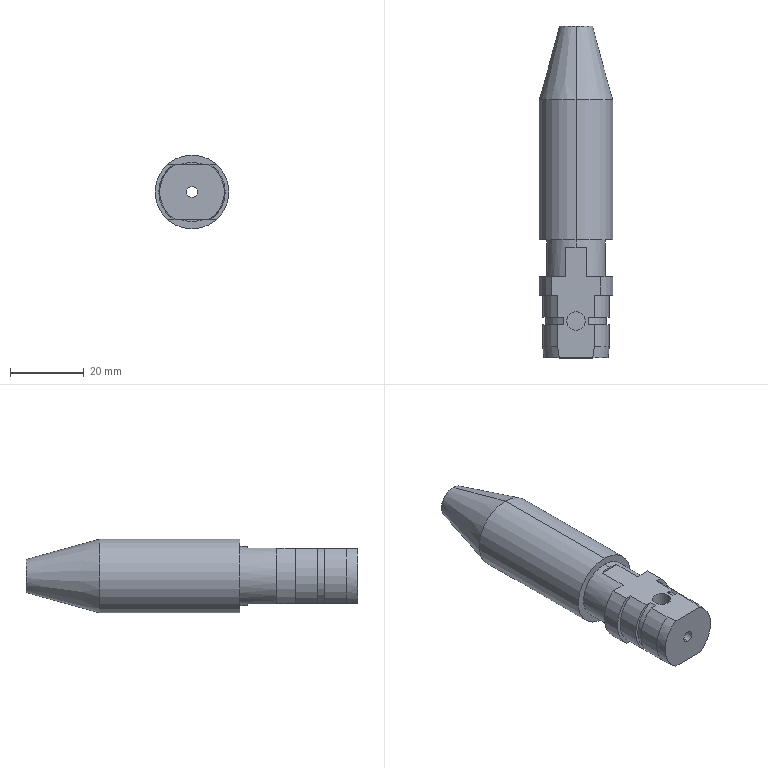Part | SolidWorks | features ICE 3, Revolution 1 | 1 solid | 39 faces | box 20 x 90 x 20 mm | volume 21802 mm3 | cylinder 18 | plane 17 | cone 4 | commonest cylinder face diameters 5 x4 18 x4 20 x4 3 x2 16 x2 16.4 x2
STEP:
#1=CARTESIAN_POINT('',(2.5,-35.854,-2.5));
#2=VERTEX_POINT('',#1);
#3=CARTESIAN_POINT('',(-2.5,-35.854,-2.5));
#4=VERTEX_POINT('',#3);
#5=CARTESIAN_POINT('',(0.,-35.854,-2.5));
#6=DIRECTION('',(0.,0.,-1.));
#7=DIRECTION('',(-1.,0.,0.));
#8=AXIS2_PLACEMENT_3D('',#5,#6,#7);
#9=CIRCLE('',#8,2.5);
#10=EDGE_CURVE('',#2,#4,#9,.T.);
#11=ORIENTED_EDGE('',*,*,#10,.F.);
#12=CARTESIAN_POINT('',(2.5,-35.854,-7.5));
#13=VERTEX_POINT('',#12);
#14=CARTESIAN_POINT('',(2.5,-35.854,-2.5));
#15=DIRECTION('',(0.,0.,-1.));
#16=VECTOR('',#15,1000.);
#17=LINE('',#14,#16);
#18=EDGE_CURVE('',#2,#13,#17,.T.);
#19=ORIENTED_EDGE('',*,*,#18,.T.);
#20=CARTESIAN_POINT('',(-2.5,-35.854,-7.5));
#21=VERTEX_POINT('',#20);
#22=CARTESIAN_POINT('',(0.,-35.854,-7.5));
#23=DIRECTION('',(0.,0.,-1.));
#24=DIRECTION('',(-1.,0.,0.));
#25=AXIS2_PLACEMENT_3D('',#22,#23,#24);
#26=CIRCLE('',#25,2.5);
#27=EDGE_CURVE('',#13,#21,#26,.T.);
#28=ORIENTED_EDGE('',*,*,#27,.T.);
#29=CARTESIAN_POINT('',(-2.5,-35.854,-2.5));
#30=DIRECTION('',(0.,0.,-1.));
#31=VECTOR('',#30,1000.);
#32=LINE('',#29,#31);
#33=EDGE_CURVE('',#4,#21,#32,.T.);
#34=ORIENTED_EDGE('',*,*,#33,.F.);
#35=EDGE_LOOP('',(#11,#19,#28,#34));
#36=FACE_OUTER_BOUND('',#35,.T.);
#37=CARTESIAN_POINT('',(0.,-35.854,-2.5));
#38=DIRECTION('',(0.,0.,-1.));
#39=DIRECTION('',(-1.,0.,0.));
#40=AXIS2_PLACEMENT_3D('',#37,#38,#39);
#41=CYLINDRICAL_SURFACE('',#40,2.5);
#42=ADVANCED_FACE('',(#36),#41,.F.);
#43=CARTESIAN_POINT('',(-2.5,-35.854,2.5));
#44=VERTEX_POINT('',#43);
#45=CARTESIAN_POINT('',(2.5,-35.854,2.5));
#46=VERTEX_POINT('',#45);
#47=CARTESIAN_POINT('',(0.,-35.854,2.5));
#48=DIRECTION('',(0.,0.,1.));
#49=DIRECTION('',(1.,0.,0.));
#50=AXIS2_PLACEMENT_3D('',#47,#48,#49);
#51=CIRCLE('',#50,2.5);
#52=EDGE_CURVE('',#44,#46,#51,.T.);
#53=ORIENTED_EDGE('',*,*,#52,.F.);
#54=CARTESIAN_POINT('',(-2.5,-35.854,7.5));
#55=VERTEX_POINT('',#54);
#56=CARTESIAN_POINT('',(-2.5,-35.854,2.5));
#57=DIRECTION('',(0.,0.,1.));
#58=VECTOR('',#57,1000.);
#59=LINE('',#56,#58);
#60=EDGE_CURVE('',#44,#55,#59,.T.);
#61=ORIENTED_EDGE('',*,*,#60,.T.);
#62=CARTESIAN_POINT('',(2.5,-35.854,7.5));
#63=VERTEX_POINT('',#62);
#64=CARTESIAN_POINT('',(0.,-35.854,7.5));
#65=DIRECTION('',(0.,0.,1.));
#66=DIRECTION('',(1.,0.,0.));
#67=AXIS2_PLACEMENT_3D('',#64,#65,#66);
#68=CIRCLE('',#67,2.5);
#69=EDGE_CURVE('',#55,#63,#68,.T.);
#70=ORIENTED_EDGE('',*,*,#69,.T.);
#71=CARTESIAN_POINT('',(2.5,-35.854,2.5));
#72=DIRECTION('',(0.,0.,1.));
#73=VECTOR('',#72,1000.);
#74=LINE('',#71,#73);
#75=EDGE_CURVE('',#46,#63,#74,.T.);
#76=ORIENTED_EDGE('',*,*,#75,.F.);
#77=EDGE_LOOP('',(#53,#61,#70,#76));
#78=FACE_OUTER_BOUND('',#77,.T.);
#79=CARTESIAN_POINT('',(0.,-35.854,2.5));
#80=DIRECTION('',(0.,0.,1.));
#81=DIRECTION('',(1.,0.,0.));
#82=AXIS2_PLACEMENT_3D('',#79,#80,#81);
#83=CYLINDRICAL_SURFACE('',#82,2.5);
#84=ADVANCED_FACE('',(#78),#83,.F.);
#85=CARTESIAN_POINT('',(0.,24.146,-10.));
#86=VERTEX_POINT('',#85);
#87=CARTESIAN_POINT('',(0.,24.146,10.));
#88=VERTEX_POINT('',#87);
#89=CARTESIAN_POINT('',(0.,24.146,0.));
#90=DIRECTION('',(0.,-1.,0.));
#91=DIRECTION('',(0.,0.,-1.));
#92=AXIS2_PLACEMENT_3D('',#89,#90,#91);
#93=CIRCLE('',#92,10.);
#94=EDGE_CURVE('',#86,#88,#93,.T.);
#95=ORIENTED_EDGE('',*,*,#94,.T.);
#96=CARTESIAN_POINT('',(0.,-13.854,10.));
#97=VERTEX_POINT('',#96);
#98=CARTESIAN_POINT('',(0.,0.,10.));
#99=DIRECTION('',(0.,-1.,0.));
#100=VECTOR('',#99,1000.);
#101=LINE('',#98,#100);
#102=EDGE_CURVE('',#88,#97,#101,.T.);
#103=ORIENTED_EDGE('',*,*,#102,.T.);
#104=CARTESIAN_POINT('',(0.,-13.854,-10.));
#105=VERTEX_POINT('',#104);
#106=CARTESIAN_POINT('',(0.,-13.854,0.));
#107=DIRECTION('',(0.,-1.,0.));
#108=DIRECTION('',(0.,0.,-1.));
#109=AXIS2_PLACEMENT_3D('',#106,#107,#108);
#110=CIRCLE('',#109,10.);
#111=EDGE_CURVE('',#105,#97,#110,.T.);
#112=ORIENTED_EDGE('',*,*,#111,.F.);
#113=CARTESIAN_POINT('',(0.,0.,-10.));
#114=DIRECTION('',(0.,-1.,0.));
#115=VECTOR('',#114,1000.);
#116=LINE('',#113,#115);
#117=EDGE_CURVE('',#86,#105,#116,.T.);
#118=ORIENTED_EDGE('',*,*,#117,.F.);
#119=EDGE_LOOP('',(#95,#103,#112,#118));
#120=FACE_OUTER_BOUND('',#119,.T.);
#121=CARTESIAN_POINT('',(0.,0.,0.));
#122=DIRECTION('',(0.,-1.,0.));
#123=DIRECTION('',(0.,0.,-1.));
#124=AXIS2_PLACEMENT_3D('',#121,#122,#123);
#125=CYLINDRICAL_SURFACE('',#124,10.);
#126=ADVANCED_FACE('',(#120),#125,.T.);
#127=CARTESIAN_POINT('',(0.,44.146,-4.5));
#128=VERTEX_POINT('',#127);
#129=CARTESIAN_POINT('',(0.,44.146,4.5));
#130=VERTEX_POINT('',#129);
#131=CARTESIAN_POINT('',(0.,44.146,0.));
#132=DIRECTION('',(0.,-1.,0.));
#133=DIRECTION('',(0.,0.,-1.));
#134=AXIS2_PLACEMENT_3D('',#131,#132,#133);
#135=CIRCLE('',#134,4.5);
#136=EDGE_CURVE('',#128,#130,#135,.T.);
#137=ORIENTED_EDGE('',*,*,#136,.T.);
#138=CARTESIAN_POINT('',(0.,44.146,4.5));
#139=DIRECTION('',(0.,-0.9642,0.2652));
#140=VECTOR('',#139,1000.);
#141=LINE('',#138,#140);
#142=EDGE_CURVE('',#130,#88,#141,.T.);
#143=ORIENTED_EDGE('',*,*,#142,.T.);
#144=ORIENTED_EDGE('',*,*,#94,.F.);
#145=CARTESIAN_POINT('',(0.,44.146,-4.5));
#146=DIRECTION('',(0.,-0.9642,-0.2652));
#147=VECTOR('',#146,1000.);
#148=LINE('',#145,#147);
#149=EDGE_CURVE('',#128,#86,#148,.T.);
#150=ORIENTED_EDGE('',*,*,#149,.F.);
#151=EDGE_LOOP('',(#137,#143,#144,#150));
#152=FACE_OUTER_BOUND('',#151,.T.);
#153=CARTESIAN_POINT('',(0.,44.146,0.));
#154=DIRECTION('',(0.,-1.,0.));
#155=DIRECTION('',(0.,0.,-1.));
#156=AXIS2_PLACEMENT_3D('',#153,#154,#155);
#157=CONICAL_SURFACE('',#156,4.5,0.2684);
#158=ADVANCED_FACE('',(#152),#157,.T.);
#159=CARTESIAN_POINT('',(0.,44.146,1.5));
#160=VERTEX_POINT('',#159);
#161=CARTESIAN_POINT('',(0.,44.146,-1.5));
#162=VERTEX_POINT('',#161);
#163=CARTESIAN_POINT('',(0.,44.146,0.));
#164=DIRECTION('',(0.,-1.,0.));
#165=DIRECTION('',(0.,0.,-1.));
#166=AXIS2_PLACEMENT_3D('',#163,#164,#165);
#167=CIRCLE('',#166,1.5);
#168=EDGE_CURVE('',#160,#162,#167,.T.);
#169=ORIENTED_EDGE('',*,*,#168,.F.);
#170=CARTESIAN_POINT('',(0.,-45.854,1.5));
#171=VERTEX_POINT('',#170);
#172=CARTESIAN_POINT('',(0.,0.,1.5));
#173=DIRECTION('',(0.,-1.,0.));
#174=VECTOR('',#173,1000.);
#175=LINE('',#172,#174);
#176=EDGE_CURVE('',#160,#171,#175,.T.);
#177=ORIENTED_EDGE('',*,*,#176,.T.);
#178=CARTESIAN_POINT('',(0.,-45.854,-1.5));
#179=VERTEX_POINT('',#178);
#180=CARTESIAN_POINT('',(0.,-45.854,0.));
#181=DIRECTION('',(0.,-1.,0.));
#182=DIRECTION('',(0.,0.,-1.));
#183=AXIS2_PLACEMENT_3D('',#180,#181,#182);
#184=CIRCLE('',#183,1.5);
#185=EDGE_CURVE('',#171,#179,#184,.T.);
#186=ORIENTED_EDGE('',*,*,#185,.T.);
#187=CARTESIAN_POINT('',(0.,0.,-1.5));
#188=DIRECTION('',(0.,-1.,0.));
#189=VECTOR('',#188,1000.);
#190=LINE('',#187,#189);
#191=EDGE_CURVE('',#162,#179,#190,.T.);
#192=ORIENTED_EDGE('',*,*,#191,.F.);
#193=EDGE_LOOP('',(#169,#177,#186,#192));
#194=FACE_OUTER_BOUND('',#193,.T.);
#195=CARTESIAN_POINT('',(0.,0.,0.));
#196=DIRECTION('',(0.,-1.,0.));
#197=DIRECTION('',(0.,0.,-1.));
#198=AXIS2_PLACEMENT_3D('',#195,#196,#197);
#199=CYLINDRICAL_SURFACE('',#198,1.5);
#200=ADVANCED_FACE('',(#194),#199,.F.);
#201=CARTESIAN_POINT('',(0.,-13.854,-8.));
#202=VERTEX_POINT('',#201);
#203=CARTESIAN_POINT('',(0.,-13.854,8.));
#204=VERTEX_POINT('',#203);
#205=CARTESIAN_POINT('',(0.,-13.854,0.));
#206=DIRECTION('',(0.,-1.,0.));
#207=DIRECTION('',(0.,0.,-1.));
#208=AXIS2_PLACEMENT_3D('',#205,#206,#207);
#209=CIRCLE('',#208,8.);
#210=EDGE_CURVE('',#202,#204,#209,.T.);
#211=ORIENTED_EDGE('',*,*,#210,.T.);
#212=CARTESIAN_POINT('',(0.,-15.854,8.));
#213=VERTEX_POINT('',#212);
#214=CARTESIAN_POINT('',(0.,0.,8.));
#215=DIRECTION('',(0.,-1.,0.));
#216=VECTOR('',#215,1000.);
#217=LINE('',#214,#216);
#218=EDGE_CURVE('',#204,#213,#217,.T.);
#219=ORIENTED_EDGE('',*,*,#218,.T.);
#220=CARTESIAN_POINT('',(2.784,-15.854,7.5));
#221=VERTEX_POINT('',#220);
#222=CARTESIAN_POINT('',(0.,-15.854,0.));
#223=DIRECTION('',(0.,-1.,0.));
#224=DIRECTION('',(0.,0.,-1.));
#225=AXIS2_PLACEMENT_3D('',#222,#223,#224);
#226=CIRCLE('',#225,8.);
#227=EDGE_CURVE('',#221,#213,#226,.T.);
#228=ORIENTED_EDGE('',*,*,#227,.F.);
#229=CARTESIAN_POINT('',(2.784,-23.854,7.5));
#230=VERTEX_POINT('',#229);
#231=CARTESIAN_POINT('',(2.784,0.,7.5));
#232=DIRECTION('',(0.,1.,0.));
#233=VECTOR('',#232,1000.);
#234=LINE('',#231,#233);
#235=EDGE_CURVE('',#230,#221,#234,.T.);
#236=ORIENTED_EDGE('',*,*,#235,.F.);
#237=CARTESIAN_POINT('',(2.784,-23.854,-7.5));
#238=VERTEX_POINT('',#237);
#239=CARTESIAN_POINT('',(0.,-23.854,0.));
#240=DIRECTION('',(0.,-1.,0.));
#241=DIRECTION('',(0.,0.,-1.));
#242=AXIS2_PLACEMENT_3D('',#239,#240,#241);
#243=CIRCLE('',#242,8.);
#244=EDGE_CURVE('',#238,#230,#243,.T.);
#245=ORIENTED_EDGE('',*,*,#244,.F.);
#246=CARTESIAN_POINT('',(2.784,-15.854,-7.5));
#247=VERTEX_POINT('',#246);
#248=CARTESIAN_POINT('',(2.784,0.,-7.5));
#249=DIRECTION('',(0.,-1.,0.));
#250=VECTOR('',#249,1000.);
#251=LINE('',#248,#250);
#252=EDGE_CURVE('',#247,#238,#251,.T.);
#253=ORIENTED_EDGE('',*,*,#252,.F.);
#254=CARTESIAN_POINT('',(0.,-15.854,-8.));
#255=VERTEX_POINT('',#254);
#256=CARTESIAN_POINT('',(0.,-15.854,0.));
#257=DIRECTION('',(0.,-1.,0.));
#258=DIRECTION('',(0.,0.,-1.));
#259=AXIS2_PLACEMENT_3D('',#256,#257,#258);
#260=CIRCLE('',#259,8.);
#261=EDGE_CURVE('',#255,#247,#260,.T.);
#262=ORIENTED_EDGE('',*,*,#261,.F.);
#263=CARTESIAN_POINT('',(0.,0.,-8.));
#264=DIRECTION('',(0.,-1.,0.));
#265=VECTOR('',#264,1000.);
#266=LINE('',#263,#265);
#267=EDGE_CURVE('',#202,#255,#266,.T.);
#268=ORIENTED_EDGE('',*,*,#267,.F.);
#269=EDGE_LOOP('',(#211,#219,#228,#236,#245,#253,#262,#268));
#270=FACE_OUTER_BOUND('',#269,.T.);
#271=CARTESIAN_POINT('',(0.,0.,0.));
#272=DIRECTION('',(0.,-1.,0.));
#273=DIRECTION('',(0.,0.,-1.));
#274=AXIS2_PLACEMENT_3D('',#271,#272,#273);
#275=CYLINDRICAL_SURFACE('',#274,8.);
#276=ADVANCED_FACE('',(#270),#275,.T.);
#277=CARTESIAN_POINT('',(0.,-45.854,0.));
#278=DIRECTION('',(0.,-1.,0.));
#279=DIRECTION('',(0.,0.,-1.));
#280=AXIS2_PLACEMENT_3D('',#277,#278,#279);
#281=CIRCLE('',#280,1.5);
#282=EDGE_CURVE('',#179,#171,#281,.T.);
#283=ORIENTED_EDGE('',*,*,#282,.F.);
#284=ORIENTED_EDGE('',*,*,#185,.F.);
#285=EDGE_LOOP('',(#283,#284));
#286=FACE_BOUND('',#285,.T.);
#287=CARTESIAN_POINT('',(-4.55,-45.854,-7.5));
#288=VERTEX_POINT('',#287);
#289=CARTESIAN_POINT('',(4.55,-45.854,-7.5));
#290=VERTEX_POINT('',#289);
#291=CARTESIAN_POINT('',(-13.155,-45.854,-7.5));
#292=DIRECTION('',(1.,0.,0.));
#293=VECTOR('',#292,1000.);
#294=LINE('',#291,#293);
#295=EDGE_CURVE('',#288,#290,#294,.T.);
#296=ORIENTED_EDGE('',*,*,#295,.T.);
#297=CARTESIAN_POINT('',(4.55,-45.854,7.5));
#298=VERTEX_POINT('',#297);
#299=CARTESIAN_POINT('',(0.,-45.854,0.));
#300=DIRECTION('',(0.,-1.,0.));
#301=DIRECTION('',(0.,0.,-1.));
#302=AXIS2_PLACEMENT_3D('',#299,#300,#301);
#303=CIRCLE('',#302,8.772);
#304=EDGE_CURVE('',#290,#298,#303,.T.);
#305=ORIENTED_EDGE('',*,*,#304,.T.);
#306=CARTESIAN_POINT('',(-4.55,-45.854,7.5));
#307=VERTEX_POINT('',#306);
#308=CARTESIAN_POINT('',(-13.155,-45.854,7.5));
#309=DIRECTION('',(-1.,0.,0.));
#310=VECTOR('',#309,1000.);
#311=LINE('',#308,#310);
#312=EDGE_CURVE('',#298,#307,#311,.T.);
#313=ORIENTED_EDGE('',*,*,#312,.T.);
#314=CARTESIAN_POINT('',(0.,-45.854,0.));
#315=DIRECTION('',(0.,-1.,0.));
#316=DIRECTION('',(0.,0.,-1.));
#317=AXIS2_PLACEMENT_3D('',#314,#315,#316);
#318=CIRCLE('',#317,8.772);
#319=EDGE_CURVE('',#307,#288,#318,.T.);
#320=ORIENTED_EDGE('',*,*,#319,.T.);
#321=EDGE_LOOP('',(#296,#305,#313,#320));
#322=FACE_OUTER_BOUND('',#321,.T.);
#323=CARTESIAN_POINT('',(-8.772,-45.854,0.));
#324=DIRECTION('',(0.,1.,0.));
#325=DIRECTION('',(0.,0.,1.));
#326=AXIS2_PLACEMENT_3D('',#323,#324,#325);
#327=PLANE('',#326);
#328=ADVANCED_FACE('',(#286,#322),#327,.F.);
#329=ORIENTED_EDGE('',*,*,#218,.F.);
#330=CARTESIAN_POINT('',(0.,-13.854,0.));
#331=DIRECTION('',(0.,-1.,0.));
#332=DIRECTION('',(0.,0.,-1.));
#333=AXIS2_PLACEMENT_3D('',#330,#331,#332);
#334=CIRCLE('',#333,8.);
#335=EDGE_CURVE('',#204,#202,#334,.T.);
#336=ORIENTED_EDGE('',*,*,#335,.T.);
#337=ORIENTED_EDGE('',*,*,#267,.T.);
#338=CARTESIAN_POINT('',(-2.784,-15.854,-7.5));
#339=VERTEX_POINT('',#338);
#340=CARTESIAN_POINT('',(0.,-15.854,0.));
#341=DIRECTION('',(0.,-1.,0.));
#342=DIRECTION('',(0.,0.,-1.));
#343=AXIS2_PLACEMENT_3D('',#340,#341,#342);
#344=CIRCLE('',#343,8.);
#345=EDGE_CURVE('',#339,#255,#344,.T.);
#346=ORIENTED_EDGE('',*,*,#345,.F.);
#347=CARTESIAN_POINT('',(-2.784,-23.854,-7.5));
#348=VERTEX_POINT('',#347);
#349=CARTESIAN_POINT('',(-2.784,0.,-7.5));
#350=DIRECTION('',(0.,1.,0.));
#351=VECTOR('',#350,1000.);
#352=LINE('',#349,#351);
#353=EDGE_CURVE('',#348,#339,#352,.T.);
#354=ORIENTED_EDGE('',*,*,#353,.F.);
#355=CARTESIAN_POINT('',(-2.784,-23.854,7.5));
#356=VERTEX_POINT('',#355);
#357=CARTESIAN_POINT('',(0.,-23.854,0.));
#358=DIRECTION('',(0.,-1.,0.));
#359=DIRECTION('',(0.,0.,-1.));
#360=AXIS2_PLACEMENT_3D('',#357,#358,#359);
#361=CIRCLE('',#360,8.);
#362=EDGE_CURVE('',#356,#348,#361,.T.);
#363=ORIENTED_EDGE('',*,*,#362,.F.);
#364=CARTESIAN_POINT('',(-2.784,-15.854,7.5));
#365=VERTEX_POINT('',#364);
#366=CARTESIAN_POINT('',(-2.784,0.,7.5));
#367=DIRECTION('',(0.,-1.,0.));
#368=VECTOR('',#367,1000.);
#369=LINE('',#366,#368);
#370=EDGE_CURVE('',#365,#356,#369,.T.);
#371=ORIENTED_EDGE('',*,*,#370,.F.);
#372=CARTESIAN_POINT('',(0.,-15.854,0.));
#373=DIRECTION('',(0.,-1.,0.));
#374=DIRECTION('',(0.,0.,-1.));
#375=AXIS2_PLACEMENT_3D('',#372,#373,#374);
#376=CIRCLE('',#375,8.);
#377=EDGE_CURVE('',#213,#365,#376,.T.);
#378=ORIENTED_EDGE('',*,*,#377,.F.);
#379=EDGE_LOOP('',(#329,#336,#337,#346,#354,#363,#371,#378));
#380=FACE_OUTER_BOUND('',#379,.T.);
#381=CARTESIAN_POINT('',(0.,0.,0.));
#382=DIRECTION('',(0.,-1.,0.));
#383=DIRECTION('',(0.,0.,-1.));
#384=AXIS2_PLACEMENT_3D('',#381,#382,#383);
#385=CYLINDRICAL_SURFACE('',#384,8.);
#386=ADVANCED_FACE('',(#380),#385,.T.);
#387=CARTESIAN_POINT('',(-6.614,-23.854,-7.5));
#388=VERTEX_POINT('',#387);
#389=CARTESIAN_POINT('',(-10.,-23.854,-7.5));
#390=DIRECTION('',(1.,0.,0.));
#391=VECTOR('',#390,1000.);
#392=LINE('',#389,#391);
#393=EDGE_CURVE('',#388,#348,#392,.T.);
#394=ORIENTED_EDGE('',*,*,#393,.F.);
#395=CARTESIAN_POINT('',(-6.614,-23.854,7.5));
#396=VERTEX_POINT('',#395);
#397=CARTESIAN_POINT('',(0.,-23.854,0.));
#398=DIRECTION('',(0.,-1.,0.));
#399=DIRECTION('',(0.,0.,-1.));
#400=AXIS2_PLACEMENT_3D('',#397,#398,#399);
#401=CIRCLE('',#400,10.);
#402=EDGE_CURVE('',#396,#388,#401,.T.);
#403=ORIENTED_EDGE('',*,*,#402,.F.);
#404=CARTESIAN_POINT('',(-10.,-23.854,7.5));
#405=DIRECTION('',(-1.,0.,0.));
#406=VECTOR('',#405,1000.);
#407=LINE('',#404,#406);
#408=EDGE_CURVE('',#356,#396,#407,.T.);
#409=ORIENTED_EDGE('',*,*,#408,.F.);
#410=ORIENTED_EDGE('',*,*,#362,.T.);
#411=EDGE_LOOP('',(#394,#403,#409,#410));
#412=FACE_OUTER_BOUND('',#411,.T.);
#413=CARTESIAN_POINT('',(-10.,-23.854,0.));
#414=DIRECTION('',(0.,-1.,0.));
#415=DIRECTION('',(0.,0.,-1.));
#416=AXIS2_PLACEMENT_3D('',#413,#414,#415);
#417=PLANE('',#416);
#418=ADVANCED_FACE('',(#412),#417,.F.);
#419=CARTESIAN_POINT('',(6.614,-23.854,-7.5));
#420=VERTEX_POINT('',#419);
#421=CARTESIAN_POINT('',(-10.,-23.854,-7.5));
#422=DIRECTION('',(1.,0.,0.));
#423=VECTOR('',#422,1000.);
#424=LINE('',#421,#423);
#425=EDGE_CURVE('',#238,#420,#424,.T.);
#426=ORIENTED_EDGE('',*,*,#425,.F.);
#427=ORIENTED_EDGE('',*,*,#244,.T.);
#428=CARTESIAN_POINT('',(6.614,-23.854,7.5));
#429=VERTEX_POINT('',#428);
#430=CARTESIAN_POINT('',(-10.,-23.854,7.5));
#431=DIRECTION('',(-1.,0.,0.));
#432=VECTOR('',#431,1000.);
#433=LINE('',#430,#432);
#434=EDGE_CURVE('',#429,#230,#433,.T.);
#435=ORIENTED_EDGE('',*,*,#434,.F.);
#436=CARTESIAN_POINT('',(0.,-23.854,0.));
#437=DIRECTION('',(0.,-1.,0.));
#438=DIRECTION('',(0.,0.,-1.));
#439=AXIS2_PLACEMENT_3D('',#436,#437,#438);
#440=CIRCLE('',#439,10.);
#441=EDGE_CURVE('',#420,#429,#440,.T.);
#442=ORIENTED_EDGE('',*,*,#441,.F.);
#443=EDGE_LOOP('',(#426,#427,#435,#442));
#444=FACE_OUTER_BOUND('',#443,.T.);
#445=CARTESIAN_POINT('',(-10.,-23.854,0.));
#446=DIRECTION('',(0.,-1.,0.));
#447=DIRECTION('',(0.,0.,-1.));
#448=AXIS2_PLACEMENT_3D('',#445,#446,#447);
#449=PLANE('',#448);
#450=ADVANCED_FACE('',(#444),#449,.F.);
#451=CARTESIAN_POINT('',(6.614,-28.854,-7.5));
#452=VERTEX_POINT('',#451);
#453=CARTESIAN_POINT('',(6.614,0.,-7.5));
#454=DIRECTION('',(0.,-1.,0.));
#455=VECTOR('',#454,1000.);
#456=LINE('',#453,#455);
#457=EDGE_CURVE('',#420,#452,#456,.T.);
#458=ORIENTED_EDGE('',*,*,#457,.F.);
#459=ORIENTED_EDGE('',*,*,#441,.T.);
#460=CARTESIAN_POINT('',(6.614,-28.854,7.5));
#461=VERTEX_POINT('',#460);
#462=CARTESIAN_POINT('',(6.614,0.,7.5));
#463=DIRECTION('',(0.,1.,0.));
#464=VECTOR('',#463,1000.);
#465=LINE('',#462,#464);
#466=EDGE_CURVE('',#461,#429,#465,.T.);
#467=ORIENTED_EDGE('',*,*,#466,.F.);
#468=CARTESIAN_POINT('',(0.,-28.854,0.));
#469=DIRECTION('',(0.,-1.,0.));
#470=DIRECTION('',(0.,0.,-1.));
#471=AXIS2_PLACEMENT_3D('',#468,#469,#470);
#472=CIRCLE('',#471,10.);
#473=EDGE_CURVE('',#452,#461,#472,.T.);
#474=ORIENTED_EDGE('',*,*,#473,.F.);
#475=EDGE_LOOP('',(#458,#459,#467,#474));
#476=FACE_OUTER_BOUND('',#475,.T.);
#477=CARTESIAN_POINT('',(0.,0.,0.));
#478=DIRECTION('',(0.,-1.,0.));
#479=DIRECTION('',(0.,0.,-1.));
#480=AXIS2_PLACEMENT_3D('',#477,#478,#479);
#481=CYLINDRICAL_SURFACE('',#480,10.);
#482=ADVANCED_FACE('',(#476),#481,.T.);
#483=CARTESIAN_POINT('',(-6.614,-28.854,-7.5));
#484=VERTEX_POINT('',#483);
#485=CARTESIAN_POINT('',(-6.614,0.,-7.5));
#486=DIRECTION('',(0.,1.,0.));
#487=VECTOR('',#486,1000.);
#488=LINE('',#485,#487);
#489=EDGE_CURVE('',#484,#388,#488,.T.);
#490=ORIENTED_EDGE('',*,*,#489,.F.);
#491=CARTESIAN_POINT('',(-6.614,-28.854,7.5));
#492=VERTEX_POINT('',#491);
#493=CARTESIAN_POINT('',(0.,-28.854,0.));
#494=DIRECTION('',(0.,-1.,0.));
#495=DIRECTION('',(0.,0.,-1.));
#496=AXIS2_PLACEMENT_3D('',#493,#494,#495);
#497=CIRCLE('',#496,10.);
#498=EDGE_CURVE('',#492,#484,#497,.T.);
#499=ORIENTED_EDGE('',*,*,#498,.F.);
#500=CARTESIAN_POINT('',(-6.614,0.,7.5));
#501=DIRECTION('',(0.,-1.,0.));
#502=VECTOR('',#501,1000.);
#503=LINE('',#500,#502);
#504=EDGE_CURVE('',#396,#492,#503,.T.);
#505=ORIENTED_EDGE('',*,*,#504,.F.);
#506=ORIENTED_EDGE('',*,*,#402,.T.);
#507=EDGE_LOOP('',(#490,#499,#505,#506));
#508=FACE_OUTER_BOUND('',#507,.T.);
#509=CARTESIAN_POINT('',(0.,0.,0.));
#510=DIRECTION('',(0.,-1.,0.));
#511=DIRECTION('',(0.,0.,-1.));
#512=AXIS2_PLACEMENT_3D('',#509,#510,#511);
#513=CYLINDRICAL_SURFACE('',#512,10.);
#514=ADVANCED_FACE('',(#508),#513,.T.);
#515=CARTESIAN_POINT('',(4.975,-28.854,-7.5));
#516=VERTEX_POINT('',#515);
#517=CARTESIAN_POINT('',(-10.,-28.854,-7.5));
#518=DIRECTION('',(-1.,0.,0.));
#519=VECTOR('',#518,1000.);
#520=LINE('',#517,#519);
#521=EDGE_CURVE('',#452,#516,#520,.T.);
#522=ORIENTED_EDGE('',*,*,#521,.F.);
#523=ORIENTED_EDGE('',*,*,#473,.T.);
#524=CARTESIAN_POINT('',(4.975,-28.854,7.5));
#525=VERTEX_POINT('',#524);
#526=CARTESIAN_POINT('',(-10.,-28.854,7.5));
#527=DIRECTION('',(1.,0.,0.));
#528=VECTOR('',#527,1000.);
#529=LINE('',#526,#528);
#530=EDGE_CURVE('',#525,#461,#529,.T.);
#531=ORIENTED_EDGE('',*,*,#530,.F.);
#532=CARTESIAN_POINT('',(0.,-28.854,0.));
#533=DIRECTION('',(0.,-1.,0.));
#534=DIRECTION('',(0.,0.,-1.));
#535=AXIS2_PLACEMENT_3D('',#532,#533,#534);
#536=CIRCLE('',#535,9.);
#537=EDGE_CURVE('',#516,#525,#536,.T.);
#538=ORIENTED_EDGE('',*,*,#537,.F.);
#539=EDGE_LOOP('',(#522,#523,#531,#538));
#540=FACE_OUTER_BOUND('',#539,.T.);
#541=CARTESIAN_POINT('',(-10.,-28.854,0.));
#542=DIRECTION('',(0.,1.,0.));
#543=DIRECTION('',(0.,0.,1.));
#544=AXIS2_PLACEMENT_3D('',#541,#542,#543);
#545=PLANE('',#544);
#546=ADVANCED_FACE('',(#540),#545,.F.);
#547=CARTESIAN_POINT('',(-4.975,-28.854,-7.5));
#548=VERTEX_POINT('',#547);
#549=CARTESIAN_POINT('',(-10.,-28.854,-7.5));
#550=DIRECTION('',(-1.,0.,0.));
#551=VECTOR('',#550,1000.);
#552=LINE('',#549,#551);
#553=EDGE_CURVE('',#548,#484,#552,.T.);
#554=ORIENTED_EDGE('',*,*,#553,.F.);
#555=CARTESIAN_POINT('',(-4.975,-28.854,7.5));
#556=VERTEX_POINT('',#555);
#557=CARTESIAN_POINT('',(0.,-28.854,0.));
#558=DIRECTION('',(0.,-1.,0.));
#559=DIRECTION('',(0.,0.,-1.));
#560=AXIS2_PLACEMENT_3D('',#557,#558,#559);
#561=CIRCLE('',#560,9.);
#562=EDGE_CURVE('',#556,#548,#561,.T.);
#563=ORIENTED_EDGE('',*,*,#562,.F.);
#564=CARTESIAN_POINT('',(-10.,-28.854,7.5));
#565=DIRECTION('',(1.,0.,0.));
#566=VECTOR('',#565,1000.);
#567=LINE('',#564,#566);
#568=EDGE_CURVE('',#492,#556,#567,.T.);
#569=ORIENTED_EDGE('',*,*,#568,.F.);
#570=ORIENTED_EDGE('',*,*,#498,.T.);
#571=EDGE_LOOP('',(#554,#563,#569,#570));
#572=FACE_OUTER_BOUND('',#571,.T.);
#573=CARTESIAN_POINT('',(-10.,-28.854,0.));
#574=DIRECTION('',(0.,1.,0.));
#575=DIRECTION('',(0.,0.,1.));
#576=AXIS2_PLACEMENT_3D('',#573,#574,#575);
#577=PLANE('',#576);
#578=ADVANCED_FACE('',(#572),#577,.F.);
#579=CARTESIAN_POINT('',(4.975,-34.854,-7.5));
#580=VERTEX_POINT('',#579);
#581=CARTESIAN_POINT('',(4.975,0.,-7.5));
#582=DIRECTION('',(0.,-1.,0.));
#583=VECTOR('',#582,1000.);
#584=LINE('',#581,#583);
#585=EDGE_CURVE('',#516,#580,#584,.T.);
#586=ORIENTED_EDGE('',*,*,#585,.F.);
#587=ORIENTED_EDGE('',*,*,#537,.T.);
#588=CARTESIAN_POINT('',(4.975,-34.854,7.5));
#589=VERTEX_POINT('',#588);
#590=CARTESIAN_POINT('',(4.975,0.,7.5));
#591=DIRECTION('',(0.,1.,0.));
#592=VECTOR('',#591,1000.);
#593=LINE('',#590,#592);
#594=EDGE_CURVE('',#589,#525,#593,.T.);
#595=ORIENTED_EDGE('',*,*,#594,.F.);
#596=CARTESIAN_POINT('',(0.,-34.854,0.));
#597=DIRECTION('',(0.,-1.,0.));
#598=DIRECTION('',(0.,0.,-1.));
#599=AXIS2_PLACEMENT_3D('',#596,#597,#598);
#600=CIRCLE('',#599,9.);
#601=EDGE_CURVE('',#580,#589,#600,.T.);
#602=ORIENTED_EDGE('',*,*,#601,.F.);
#603=EDGE_LOOP('',(#586,#587,#595,#602));
#604=FACE_OUTER_BOUND('',#603,.T.);
#605=CARTESIAN_POINT('',(0.,0.,0.));
#606=DIRECTION('',(0.,-1.,0.));
#607=DIRECTION('',(0.,0.,-1.));
#608=AXIS2_PLACEMENT_3D('',#605,#606,#607);
#609=CYLINDRICAL_SURFACE('',#608,9.);
#610=ADVANCED_FACE('',(#604),#609,.T.);
#611=CARTESIAN_POINT('',(-4.975,-34.854,-7.5));
#612=VERTEX_POINT('',#611);
#613=CARTESIAN_POINT('',(-4.975,0.,-7.5));
#614=DIRECTION('',(0.,1.,0.));
#615=VECTOR('',#614,1000.);
#616=LINE('',#613,#615);
#617=EDGE_CURVE('',#612,#548,#616,.T.);
#618=ORIENTED_EDGE('',*,*,#617,.F.);
#619=CARTESIAN_POINT('',(-4.975,-34.854,7.5));
#620=VERTEX_POINT('',#619);
#621=CARTESIAN_POINT('',(0.,-34.854,0.));
#622=DIRECTION('',(0.,-1.,0.));
#623=DIRECTION('',(0.,0.,-1.));
#624=AXIS2_PLACEMENT_3D('',#621,#622,#623);
#625=CIRCLE('',#624,9.);
#626=EDGE_CURVE('',#620,#612,#625,.T.);
#627=ORIENTED_EDGE('',*,*,#626,.F.);
#628=CARTESIAN_POINT('',(-4.975,0.,7.5));
#629=DIRECTION('',(0.,-1.,0.));
#630=VECTOR('',#629,1000.);
#631=LINE('',#628,#630);
#632=EDGE_CURVE('',#556,#620,#631,.T.);
#633=ORIENTED_EDGE('',*,*,#632,.F.);
#634=ORIENTED_EDGE('',*,*,#562,.T.);
#635=EDGE_LOOP('',(#618,#627,#633,#634));
#636=FACE_OUTER_BOUND('',#635,.T.);
#637=CARTESIAN_POINT('',(0.,0.,0.));
#638=DIRECTION('',(0.,-1.,0.));
#639=DIRECTION('',(0.,0.,-1.));
#640=AXIS2_PLACEMENT_3D('',#637,#638,#639);
#641=CYLINDRICAL_SURFACE('',#640,9.);
#642=ADVANCED_FACE('',(#636),#641,.T.);
#643=CARTESIAN_POINT('',(3.315,-34.854,-7.5));
#644=VERTEX_POINT('',#643);
#645=CARTESIAN_POINT('',(-9.,-34.854,-7.5));
#646=DIRECTION('',(-1.,0.,0.));
#647=VECTOR('',#646,1000.);
#648=LINE('',#645,#647);
#649=EDGE_CURVE('',#580,#644,#648,.T.);
#650=ORIENTED_EDGE('',*,*,#649,.F.);
#651=ORIENTED_EDGE('',*,*,#601,.T.);
#652=CARTESIAN_POINT('',(3.315,-34.854,7.5));
#653=VERTEX_POINT('',#652);
#654=CARTESIAN_POINT('',(-9.,-34.854,7.5));
#655=DIRECTION('',(1.,0.,0.));
#656=VECTOR('',#655,1000.);
#657=LINE('',#654,#656);
#658=EDGE_CURVE('',#653,#589,#657,.T.);
#659=ORIENTED_EDGE('',*,*,#658,.F.);
#660=CARTESIAN_POINT('',(0.,-34.854,0.));
#661=DIRECTION('',(0.,-1.,0.));
#662=DIRECTION('',(0.,0.,-1.));
#663=AXIS2_PLACEMENT_3D('',#660,#661,#662);
#664=CIRCLE('',#663,8.2);
#665=EDGE_CURVE('',#644,#653,#664,.T.);
#666=ORIENTED_EDGE('',*,*,#665,.F.);
#667=EDGE_LOOP('',(#650,#651,#659,#666));
#668=FACE_OUTER_BOUND('',#667,.T.);
#669=CARTESIAN_POINT('',(-9.,-34.854,0.));
#670=DIRECTION('',(0.,1.,0.));
#671=DIRECTION('',(0.,0.,1.));
#672=AXIS2_PLACEMENT_3D('',#669,#670,#671);
#673=PLANE('',#672);
#674=ADVANCED_FACE('',(#668),#673,.F.);
#675=CARTESIAN_POINT('',(-3.315,-34.854,-7.5));
#676=VERTEX_POINT('',#675);
#677=CARTESIAN_POINT('',(-9.,-34.854,-7.5));
#678=DIRECTION('',(-1.,0.,0.));
#679=VECTOR('',#678,1000.);
#680=LINE('',#677,#679);
#681=EDGE_CURVE('',#676,#612,#680,.T.);
#682=ORIENTED_EDGE('',*,*,#681,.F.);
#683=CARTESIAN_POINT('',(-3.315,-34.854,7.5));
#684=VERTEX_POINT('',#683);
#685=CARTESIAN_POINT('',(0.,-34.854,0.));
#686=DIRECTION('',(0.,-1.,0.));
#687=DIRECTION('',(0.,0.,-1.));
#688=AXIS2_PLACEMENT_3D('',#685,#686,#687);
#689=CIRCLE('',#688,8.2);
#690=EDGE_CURVE('',#684,#676,#689,.T.);
#691=ORIENTED_EDGE('',*,*,#690,.F.);
#692=CARTESIAN_POINT('',(-9.,-34.854,7.5));
#693=DIRECTION('',(1.,0.,0.));
#694=VECTOR('',#693,1000.);
#695=LINE('',#692,#694);
#696=EDGE_CURVE('',#620,#684,#695,.T.);
#697=ORIENTED_EDGE('',*,*,#696,.F.);
#698=ORIENTED_EDGE('',*,*,#626,.T.);
#699=EDGE_LOOP('',(#682,#691,#697,#698));
#700=FACE_OUTER_BOUND('',#699,.T.);
#701=CARTESIAN_POINT('',(-9.,-34.854,0.));
#702=DIRECTION('',(0.,1.,0.));
#703=DIRECTION('',(0.,0.,1.));
#704=AXIS2_PLACEMENT_3D('',#701,#702,#703);
#705=PLANE('',#704);
#706=ADVANCED_FACE('',(#700),#705,.F.);
#707=CARTESIAN_POINT('',(3.315,-36.854,-7.5));
#708=VERTEX_POINT('',#707);
#709=CARTESIAN_POINT('',(3.315,0.,-7.5));
#710=DIRECTION('',(0.,-1.,0.));
#711=VECTOR('',#710,1000.);
#712=LINE('',#709,#711);
#713=EDGE_CURVE('',#644,#708,#712,.T.);
#714=ORIENTED_EDGE('',*,*,#713,.F.);
#715=ORIENTED_EDGE('',*,*,#665,.T.);
#716=CARTESIAN_POINT('',(3.315,-36.854,7.5));
#717=VERTEX_POINT('',#716);
#718=CARTESIAN_POINT('',(3.315,0.,7.5));
#719=DIRECTION('',(0.,1.,0.));
#720=VECTOR('',#719,1000.);
#721=LINE('',#718,#720);
#722=EDGE_CURVE('',#717,#653,#721,.T.);
#723=ORIENTED_EDGE('',*,*,#722,.F.);
#724=CARTESIAN_POINT('',(0.,-36.854,0.));
#725=DIRECTION('',(0.,-1.,0.));
#726=DIRECTION('',(0.,0.,-1.));
#727=AXIS2_PLACEMENT_3D('',#724,#725,#726);
#728=CIRCLE('',#727,8.2);
#729=EDGE_CURVE('',#708,#717,#728,.T.);
#730=ORIENTED_EDGE('',*,*,#729,.F.);
#731=EDGE_LOOP('',(#714,#715,#723,#730));
#732=FACE_OUTER_BOUND('',#731,.T.);
#733=CARTESIAN_POINT('',(0.,0.,0.));
#734=DIRECTION('',(0.,-1.,0.));
#735=DIRECTION('',(0.,0.,-1.));
#736=AXIS2_PLACEMENT_3D('',#733,#734,#735);
#737=CYLINDRICAL_SURFACE('',#736,8.2);
#738=ADVANCED_FACE('',(#732),#737,.T.);
#739=CARTESIAN_POINT('',(-3.315,-36.854,-7.5));
#740=VERTEX_POINT('',#739);
#741=CARTESIAN_POINT('',(-3.315,0.,-7.5));
#742=DIRECTION('',(0.,1.,0.));
#743=VECTOR('',#742,1000.);
#744=LINE('',#741,#743);
#745=EDGE_CURVE('',#740,#676,#744,.T.);
#746=ORIENTED_EDGE('',*,*,#745,.F.);
#747=CARTESIAN_POINT('',(-3.315,-36.854,7.5));
#748=VERTEX_POINT('',#747);
#749=CARTESIAN_POINT('',(0.,-36.854,0.));
#750=DIRECTION('',(0.,-1.,0.));
#751=DIRECTION('',(0.,0.,-1.));
#752=AXIS2_PLACEMENT_3D('',#749,#750,#751);
#753=CIRCLE('',#752,8.2);
#754=EDGE_CURVE('',#748,#740,#753,.T.);
#755=ORIENTED_EDGE('',*,*,#754,.F.);
#756=CARTESIAN_POINT('',(-3.315,0.,7.5));
#757=DIRECTION('',(0.,-1.,0.));
#758=VECTOR('',#757,1000.);
#759=LINE('',#756,#758);
#760=EDGE_CURVE('',#684,#748,#759,.T.);
#761=ORIENTED_EDGE('',*,*,#760,.F.);
#762=ORIENTED_EDGE('',*,*,#690,.T.);
#763=EDGE_LOOP('',(#746,#755,#761,#762));
#764=FACE_OUTER_BOUND('',#763,.T.);
#765=CARTESIAN_POINT('',(0.,0.,0.));
#766=DIRECTION('',(0.,-1.,0.));
#767=DIRECTION('',(0.,0.,-1.));
#768=AXIS2_PLACEMENT_3D('',#765,#766,#767);
#769=CYLINDRICAL_SURFACE('',#768,8.2);
#770=ADVANCED_FACE('',(#764),#769,.T.);
#771=CARTESIAN_POINT('',(-4.975,-36.854,-7.5));
#772=VERTEX_POINT('',#771);
#773=CARTESIAN_POINT('',(-9.,-36.854,-7.5));
#774=DIRECTION('',(1.,0.,0.));
#775=VECTOR('',#774,1000.);
#776=LINE('',#773,#775);
#777=EDGE_CURVE('',#772,#740,#776,.T.);
#778=ORIENTED_EDGE('',*,*,#777,.F.);
#779=CARTESIAN_POINT('',(-4.975,-36.854,7.5));
#780=VERTEX_POINT('',#779);
#781=CARTESIAN_POINT('',(0.,-36.854,0.));
#782=DIRECTION('',(0.,-1.,0.));
#783=DIRECTION('',(0.,0.,-1.));
#784=AXIS2_PLACEMENT_3D('',#781,#782,#783);
#785=CIRCLE('',#784,9.);
#786=EDGE_CURVE('',#780,#772,#785,.T.);
#787=ORIENTED_EDGE('',*,*,#786,.F.);
#788=CARTESIAN_POINT('',(-9.,-36.854,7.5));
#789=DIRECTION('',(-1.,0.,0.));
#790=VECTOR('',#789,1000.);
#791=LINE('',#788,#790);
#792=EDGE_CURVE('',#748,#780,#791,.T.);
#793=ORIENTED_EDGE('',*,*,#792,.F.);
#794=ORIENTED_EDGE('',*,*,#754,.T.);
#795=EDGE_LOOP('',(#778,#787,#793,#794));
#796=FACE_OUTER_BOUND('',#795,.T.);
#797=CARTESIAN_POINT('',(-9.,-36.854,0.));
#798=DIRECTION('',(0.,-1.,0.));
#799=DIRECTION('',(0.,0.,-1.));
#800=AXIS2_PLACEMENT_3D('',#797,#798,#799);
#801=PLANE('',#800);
#802=ADVANCED_FACE('',(#796),#801,.F.);
#803=CARTESIAN_POINT('',(4.975,-36.854,-7.5));
#804=VERTEX_POINT('',#803);
#805=CARTESIAN_POINT('',(-9.,-36.854,-7.5));
#806=DIRECTION('',(1.,0.,0.));
#807=VECTOR('',#806,1000.);
#808=LINE('',#805,#807);
#809=EDGE_CURVE('',#708,#804,#808,.T.);
#810=ORIENTED_EDGE('',*,*,#809,.F.);
#811=ORIENTED_EDGE('',*,*,#729,.T.);
#812=CARTESIAN_POINT('',(4.975,-36.854,7.5));
#813=VERTEX_POINT('',#812);
#814=CARTESIAN_POINT('',(-9.,-36.854,7.5));
#815=DIRECTION('',(-1.,0.,0.));
#816=VECTOR('',#815,1000.);
#817=LINE('',#814,#816);
#818=EDGE_CURVE('',#813,#717,#817,.T.);
#819=ORIENTED_EDGE('',*,*,#818,.F.);
#820=CARTESIAN_POINT('',(0.,-36.854,0.));
#821=DIRECTION('',(0.,-1.,0.));
#822=DIRECTION('',(0.,0.,-1.));
#823=AXIS2_PLACEMENT_3D('',#820,#821,#822);
#824=CIRCLE('',#823,9.);
#825=EDGE_CURVE('',#804,#813,#824,.T.);
#826=ORIENTED_EDGE('',*,*,#825,.F.);
#827=EDGE_LOOP('',(#810,#811,#819,#826));
#828=FACE_OUTER_BOUND('',#827,.T.);
#829=CARTESIAN_POINT('',(-9.,-36.854,0.));
#830=DIRECTION('',(0.,-1.,0.));
#831=DIRECTION('',(0.,0.,-1.));
#832=AXIS2_PLACEMENT_3D('',#829,#830,#831);
#833=PLANE('',#832);
#834=ADVANCED_FACE('',(#828),#833,.F.);
#835=CARTESIAN_POINT('',(4.975,-42.854,-7.5));
#836=VERTEX_POINT('',#835);
#837=CARTESIAN_POINT('',(4.975,0.,-7.5));
#838=DIRECTION('',(0.,-1.,0.));
#839=VECTOR('',#838,1000.);
#840=LINE('',#837,#839);
#841=EDGE_CURVE('',#804,#836,#840,.T.);
#842=ORIENTED_EDGE('',*,*,#841,.F.);
#843=ORIENTED_EDGE('',*,*,#825,.T.);
#844=CARTESIAN_POINT('',(4.975,-42.854,7.5));
#845=VERTEX_POINT('',#844);
#846=CARTESIAN_POINT('',(4.975,0.,7.5));
#847=DIRECTION('',(0.,1.,0.));
#848=VECTOR('',#847,1000.);
#849=LINE('',#846,#848);
#850=EDGE_CURVE('',#845,#813,#849,.T.);
#851=ORIENTED_EDGE('',*,*,#850,.F.);
#852=CARTESIAN_POINT('',(0.,-42.854,0.));
#853=DIRECTION('',(0.,-1.,0.));
#854=DIRECTION('',(0.,0.,-1.));
#855=AXIS2_PLACEMENT_3D('',#852,#853,#854);
#856=CIRCLE('',#855,9.);
#857=EDGE_CURVE('',#836,#845,#856,.T.);
#858=ORIENTED_EDGE('',*,*,#857,.F.);
#859=EDGE_LOOP('',(#842,#843,#851,#858));
#860=FACE_OUTER_BOUND('',#859,.T.);
#861=CARTESIAN_POINT('',(0.,0.,0.));
#862=DIRECTION('',(0.,-1.,0.));
#863=DIRECTION('',(0.,0.,-1.));
#864=AXIS2_PLACEMENT_3D('',#861,#862,#863);
#865=CYLINDRICAL_SURFACE('',#864,9.);
#866=ADVANCED_FACE('',(#860),#865,.T.);
#867=CARTESIAN_POINT('',(-4.975,-42.854,-7.5));
#868=VERTEX_POINT('',#867);
#869=CARTESIAN_POINT('',(-4.975,0.,-7.5));
#870=DIRECTION('',(0.,1.,0.));
#871=VECTOR('',#870,1000.);
#872=LINE('',#869,#871);
#873=EDGE_CURVE('',#868,#772,#872,.T.);
#874=ORIENTED_EDGE('',*,*,#873,.F.);
#875=CARTESIAN_POINT('',(-4.975,-42.854,7.5));
#876=VERTEX_POINT('',#875);
#877=CARTESIAN_POINT('',(0.,-42.854,0.));
#878=DIRECTION('',(0.,-1.,0.));
#879=DIRECTION('',(0.,0.,-1.));
#880=AXIS2_PLACEMENT_3D('',#877,#878,#879);
#881=CIRCLE('',#880,9.);
#882=EDGE_CURVE('',#876,#868,#881,.T.);
#883=ORIENTED_EDGE('',*,*,#882,.F.);
#884=CARTESIAN_POINT('',(-4.975,0.,7.5));
#885=DIRECTION('',(0.,-1.,0.));
#886=VECTOR('',#885,1000.);
#887=LINE('',#884,#886);
#888=EDGE_CURVE('',#780,#876,#887,.T.);
#889=ORIENTED_EDGE('',*,*,#888,.F.);
#890=ORIENTED_EDGE('',*,*,#786,.T.);
#891=EDGE_LOOP('',(#874,#883,#889,#890));
#892=FACE_OUTER_BOUND('',#891,.T.);
#893=CARTESIAN_POINT('',(0.,0.,0.));
#894=DIRECTION('',(0.,-1.,0.));
#895=DIRECTION('',(0.,0.,-1.));
#896=AXIS2_PLACEMENT_3D('',#893,#894,#895);
#897=CYLINDRICAL_SURFACE('',#896,9.);
#898=ADVANCED_FACE('',(#892),#897,.T.);
#899=CARTESIAN_POINT('',(-4.55,-45.854,-7.5));
#900=CARTESIAN_POINT('',(-4.696,-44.855,-7.5));
#901=CARTESIAN_POINT('',(-4.838,-43.855,-7.5));
#902=CARTESIAN_POINT('',(-4.975,-42.854,-7.5));
#903=B_SPLINE_CURVE_WITH_KNOTS('',3,(#899,#900,#901,#902),.UNSPECIFIED.,.F.,.F.,(4,4),(0.01484,0.01787),.UNSPECIFIED.);
#904=EDGE_CURVE('',#288,#868,#903,.T.);
#905=ORIENTED_EDGE('',*,*,#904,.F.);
#906=ORIENTED_EDGE('',*,*,#319,.F.);
#907=CARTESIAN_POINT('',(-4.975,-42.854,7.5));
#908=CARTESIAN_POINT('',(-4.838,-43.855,7.5));
#909=CARTESIAN_POINT('',(-4.696,-44.855,7.5));
#910=CARTESIAN_POINT('',(-4.55,-45.854,7.5));
#911=B_SPLINE_CURVE_WITH_KNOTS('',3,(#907,#908,#909,#910),.UNSPECIFIED.,.F.,.F.,(4,4),(0.01526,0.01829),.UNSPECIFIED.);
#912=EDGE_CURVE('',#876,#307,#911,.T.);
#913=ORIENTED_EDGE('',*,*,#912,.F.);
#914=ORIENTED_EDGE('',*,*,#882,.T.);
#915=EDGE_LOOP('',(#905,#906,#913,#914));
#916=FACE_OUTER_BOUND('',#915,.T.);
#917=CARTESIAN_POINT('',(0.,-42.854,0.));
#918=DIRECTION('',(0.,1.,0.));
#919=DIRECTION('',(0.,0.,1.));
#920=AXIS2_PLACEMENT_3D('',#917,#918,#919);
#921=CONICAL_SURFACE('',#920,9.,0.07574);
#922=ADVANCED_FACE('',(#916),#921,.T.);
#923=CARTESIAN_POINT('',(4.975,-42.854,-7.5));
#924=CARTESIAN_POINT('',(4.838,-43.855,-7.5));
#925=CARTESIAN_POINT('',(4.696,-44.855,-7.5));
#926=CARTESIAN_POINT('',(4.55,-45.854,-7.5));
#927=B_SPLINE_CURVE_WITH_KNOTS('',3,(#923,#924,#925,#926),.UNSPECIFIED.,.F.,.F.,(4,4),(0.01526,0.01829),.UNSPECIFIED.);
#928=EDGE_CURVE('',#836,#290,#927,.T.);
#929=ORIENTED_EDGE('',*,*,#928,.F.);
#930=ORIENTED_EDGE('',*,*,#857,.T.);
#931=CARTESIAN_POINT('',(4.55,-45.854,7.5));
#932=CARTESIAN_POINT('',(4.696,-44.855,7.5));
#933=CARTESIAN_POINT('',(4.838,-43.855,7.5));
#934=CARTESIAN_POINT('',(4.975,-42.854,7.5));
#935=B_SPLINE_CURVE_WITH_KNOTS('',3,(#931,#932,#933,#934),.UNSPECIFIED.,.F.,.F.,(4,4),(0.01484,0.01787),.UNSPECIFIED.);
#936=EDGE_CURVE('',#298,#845,#935,.T.);
#937=ORIENTED_EDGE('',*,*,#936,.F.);
#938=ORIENTED_EDGE('',*,*,#304,.F.);
#939=EDGE_LOOP('',(#929,#930,#937,#938));
#940=FACE_OUTER_BOUND('',#939,.T.);
#941=CARTESIAN_POINT('',(0.,-42.854,0.));
#942=DIRECTION('',(0.,1.,0.));
#943=DIRECTION('',(0.,0.,1.));
#944=AXIS2_PLACEMENT_3D('',#941,#942,#943);
#945=CONICAL_SURFACE('',#944,9.,0.07574);
#946=ADVANCED_FACE('',(#940),#945,.T.);
#947=ORIENTED_EDGE('',*,*,#176,.F.);
#948=CARTESIAN_POINT('',(0.,44.146,0.));
#949=DIRECTION('',(0.,-1.,0.));
#950=DIRECTION('',(0.,0.,-1.));
#951=AXIS2_PLACEMENT_3D('',#948,#949,#950);
#952=CIRCLE('',#951,1.5);
#953=EDGE_CURVE('',#162,#160,#952,.T.);
#954=ORIENTED_EDGE('',*,*,#953,.F.);
#955=ORIENTED_EDGE('',*,*,#191,.T.);
#956=ORIENTED_EDGE('',*,*,#282,.T.);
#957=EDGE_LOOP('',(#947,#954,#955,#956));
#958=FACE_OUTER_BOUND('',#957,.T.);
#959=CARTESIAN_POINT('',(0.,0.,0.));
#960=DIRECTION('',(0.,-1.,0.));
#961=DIRECTION('',(0.,0.,-1.));
#962=AXIS2_PLACEMENT_3D('',#959,#960,#961);
#963=CYLINDRICAL_SURFACE('',#962,1.5);
#964=ADVANCED_FACE('',(#958),#963,.F.);
#965=ORIENTED_EDGE('',*,*,#136,.F.);
#966=CARTESIAN_POINT('',(0.,44.146,0.));
#967=DIRECTION('',(0.,-1.,0.));
#968=DIRECTION('',(0.,0.,-1.));
#969=AXIS2_PLACEMENT_3D('',#966,#967,#968);
#970=CIRCLE('',#969,4.5);
#971=EDGE_CURVE('',#130,#128,#970,.T.);
#972=ORIENTED_EDGE('',*,*,#971,.F.);
#973=EDGE_LOOP('',(#965,#972));
#974=FACE_OUTER_BOUND('',#973,.T.);
#975=ORIENTED_EDGE('',*,*,#953,.T.);
#976=ORIENTED_EDGE('',*,*,#168,.T.);
#977=EDGE_LOOP('',(#975,#976));
#978=FACE_BOUND('',#977,.T.);
#979=CARTESIAN_POINT('',(-1.5,44.146,0.));
#980=DIRECTION('',(0.,-1.,0.));
#981=DIRECTION('',(0.,0.,-1.));
#982=AXIS2_PLACEMENT_3D('',#979,#980,#981);
#983=PLANE('',#982);
#984=ADVANCED_FACE('',(#974,#978),#983,.F.);
#985=ORIENTED_EDGE('',*,*,#142,.F.);
#986=ORIENTED_EDGE('',*,*,#971,.T.);
#987=ORIENTED_EDGE('',*,*,#149,.T.);
#988=CARTESIAN_POINT('',(0.,24.146,0.));
#989=DIRECTION('',(0.,-1.,0.));
#990=DIRECTION('',(0.,0.,-1.));
#991=AXIS2_PLACEMENT_3D('',#988,#989,#990);
#992=CIRCLE('',#991,10.);
#993=EDGE_CURVE('',#88,#86,#992,.T.);
#994=ORIENTED_EDGE('',*,*,#993,.F.);
#995=EDGE_LOOP('',(#985,#986,#987,#994));
#996=FACE_OUTER_BOUND('',#995,.T.);
#997=CARTESIAN_POINT('',(0.,44.146,0.));
#998=DIRECTION('',(0.,-1.,0.));
#999=DIRECTION('',(0.,0.,-1.));
#1000=AXIS2_PLACEMENT_3D('',#997,#998,#999);
#1001=CONICAL_SURFACE('',#1000,4.5,0.2684);
#1002=ADVANCED_FACE('',(#996),#1001,.T.);
#1003=ORIENTED_EDGE('',*,*,#102,.F.);
#1004=ORIENTED_EDGE('',*,*,#993,.T.);
#1005=ORIENTED_EDGE('',*,*,#117,.T.);
#1006=CARTESIAN_POINT('',(0.,-13.854,0.));
#1007=DIRECTION('',(0.,-1.,0.));
#1008=DIRECTION('',(0.,0.,-1.));
#1009=AXIS2_PLACEMENT_3D('',#1006,#1007,#1008);
#1010=CIRCLE('',#1009,10.);
#1011=EDGE_CURVE('',#97,#105,#1010,.T.);
#1012=ORIENTED_EDGE('',*,*,#1011,.F.);
#1013=EDGE_LOOP('',(#1003,#1004,#1005,#1012));
#1014=FACE_OUTER_BOUND('',#1013,.T.);
#1015=CARTESIAN_POINT('',(0.,0.,0.));
#1016=DIRECTION('',(0.,-1.,0.));
#1017=DIRECTION('',(0.,0.,-1.));
#1018=AXIS2_PLACEMENT_3D('',#1015,#1016,#1017);
#1019=CYLINDRICAL_SURFACE('',#1018,10.);
#1020=ADVANCED_FACE('',(#1014),#1019,.T.);
#1021=ORIENTED_EDGE('',*,*,#210,.F.);
#1022=ORIENTED_EDGE('',*,*,#335,.F.);
#1023=EDGE_LOOP('',(#1021,#1022));
#1024=FACE_BOUND('',#1023,.T.);
#1025=ORIENTED_EDGE('',*,*,#111,.T.);
#1026=ORIENTED_EDGE('',*,*,#1011,.T.);
#1027=EDGE_LOOP('',(#1025,#1026));
#1028=FACE_OUTER_BOUND('',#1027,.T.);
#1029=CARTESIAN_POINT('',(-8.,-13.854,0.));
#1030=DIRECTION('',(0.,1.,0.));
#1031=DIRECTION('',(0.,0.,1.));
#1032=AXIS2_PLACEMENT_3D('',#1029,#1030,#1031);
#1033=PLANE('',#1032);
#1034=ADVANCED_FACE('',(#1024,#1028),#1033,.F.);
#1035=CARTESIAN_POINT('',(0.,-35.854,7.5));
#1036=DIRECTION('',(0.,0.,1.));
#1037=DIRECTION('',(1.,0.,0.));
#1038=AXIS2_PLACEMENT_3D('',#1035,#1036,#1037);
#1039=CIRCLE('',#1038,2.5);
#1040=EDGE_CURVE('',#63,#55,#1039,.T.);
#1041=ORIENTED_EDGE('',*,*,#1040,.F.);
#1042=ORIENTED_EDGE('',*,*,#69,.F.);
#1043=EDGE_LOOP('',(#1041,#1042));
#1044=FACE_BOUND('',#1043,.T.);
#1045=ORIENTED_EDGE('',*,*,#370,.T.);
#1046=ORIENTED_EDGE('',*,*,#408,.T.);
#1047=ORIENTED_EDGE('',*,*,#504,.T.);
#1048=ORIENTED_EDGE('',*,*,#568,.T.);
#1049=ORIENTED_EDGE('',*,*,#632,.T.);
#1050=ORIENTED_EDGE('',*,*,#696,.T.);
#1051=ORIENTED_EDGE('',*,*,#760,.T.);
#1052=ORIENTED_EDGE('',*,*,#792,.T.);
#1053=ORIENTED_EDGE('',*,*,#888,.T.);
#1054=ORIENTED_EDGE('',*,*,#912,.T.);
#1055=ORIENTED_EDGE('',*,*,#312,.F.);
#1056=ORIENTED_EDGE('',*,*,#936,.T.);
#1057=ORIENTED_EDGE('',*,*,#850,.T.);
#1058=ORIENTED_EDGE('',*,*,#818,.T.);
#1059=ORIENTED_EDGE('',*,*,#722,.T.);
#1060=ORIENTED_EDGE('',*,*,#658,.T.);
#1061=ORIENTED_EDGE('',*,*,#594,.T.);
#1062=ORIENTED_EDGE('',*,*,#530,.T.);
#1063=ORIENTED_EDGE('',*,*,#466,.T.);
#1064=ORIENTED_EDGE('',*,*,#434,.T.);
#1065=ORIENTED_EDGE('',*,*,#235,.T.);
#1066=CARTESIAN_POINT('',(-13.155,-15.854,7.5));
#1067=DIRECTION('',(-1.,0.,0.));
#1068=VECTOR('',#1067,1000.);
#1069=LINE('',#1066,#1068);
#1070=EDGE_CURVE('',#221,#365,#1069,.T.);
#1071=ORIENTED_EDGE('',*,*,#1070,.T.);
#1072=EDGE_LOOP('',(#1045,#1046,#1047,#1048,#1049,#1050,#1051,#1052,#1053,#1054,#1055,#1056,#1057,#1058,#1059,#1060,#1061,#1062,#1063,#1064,#1065,#1071));
#1073=FACE_OUTER_BOUND('',#1072,.T.);
#1074=CARTESIAN_POINT('',(-13.155,-15.854,7.5));
#1075=DIRECTION('',(0.,0.,1.));
#1076=DIRECTION('',(1.,0.,0.));
#1077=AXIS2_PLACEMENT_3D('',#1074,#1075,#1076);
#1078=PLANE('',#1077);
#1079=ADVANCED_FACE('',(#1044,#1073),#1078,.T.);
#1080=ORIENTED_EDGE('',*,*,#227,.T.);
#1081=ORIENTED_EDGE('',*,*,#377,.T.);
#1082=ORIENTED_EDGE('',*,*,#1070,.F.);
#1083=EDGE_LOOP('',(#1080,#1081,#1082));
#1084=FACE_OUTER_BOUND('',#1083,.T.);
#1085=CARTESIAN_POINT('',(0.,-15.854,0.));
#1086=DIRECTION('',(0.,-1.,0.));
#1087=DIRECTION('',(0.,0.,-1.));
#1088=AXIS2_PLACEMENT_3D('',#1085,#1086,#1087);
#1089=PLANE('',#1088);
#1090=ADVANCED_FACE('',(#1084),#1089,.T.);
#1091=ORIENTED_EDGE('',*,*,#345,.T.);
#1092=ORIENTED_EDGE('',*,*,#261,.T.);
#1093=CARTESIAN_POINT('',(-13.155,-15.854,-7.5));
#1094=DIRECTION('',(1.,0.,0.));
#1095=VECTOR('',#1094,1000.);
#1096=LINE('',#1093,#1095);
#1097=EDGE_CURVE('',#339,#247,#1096,.T.);
#1098=ORIENTED_EDGE('',*,*,#1097,.F.);
#1099=EDGE_LOOP('',(#1091,#1092,#1098));
#1100=FACE_OUTER_BOUND('',#1099,.T.);
#1101=CARTESIAN_POINT('',(0.,-15.854,0.));
#1102=DIRECTION('',(0.,-1.,0.));
#1103=DIRECTION('',(0.,0.,-1.));
#1104=AXIS2_PLACEMENT_3D('',#1101,#1102,#1103);
#1105=PLANE('',#1104);
#1106=ADVANCED_FACE('',(#1100),#1105,.T.);
#1107=CARTESIAN_POINT('',(0.,-35.854,-7.5));
#1108=DIRECTION('',(0.,0.,-1.));
#1109=DIRECTION('',(-1.,0.,0.));
#1110=AXIS2_PLACEMENT_3D('',#1107,#1108,#1109);
#1111=CIRCLE('',#1110,2.5);
#1112=EDGE_CURVE('',#21,#13,#1111,.T.);
#1113=ORIENTED_EDGE('',*,*,#1112,.F.);
#1114=ORIENTED_EDGE('',*,*,#27,.F.);
#1115=EDGE_LOOP('',(#1113,#1114));
#1116=FACE_BOUND('',#1115,.T.);
#1117=ORIENTED_EDGE('',*,*,#353,.T.);
#1118=ORIENTED_EDGE('',*,*,#1097,.T.);
#1119=ORIENTED_EDGE('',*,*,#252,.T.);
#1120=ORIENTED_EDGE('',*,*,#425,.T.);
#1121=ORIENTED_EDGE('',*,*,#457,.T.);
#1122=ORIENTED_EDGE('',*,*,#521,.T.);
#1123=ORIENTED_EDGE('',*,*,#585,.T.);
#1124=ORIENTED_EDGE('',*,*,#649,.T.);
#1125=ORIENTED_EDGE('',*,*,#713,.T.);
#1126=ORIENTED_EDGE('',*,*,#809,.T.);
#1127=ORIENTED_EDGE('',*,*,#841,.T.);
#1128=ORIENTED_EDGE('',*,*,#928,.T.);
#1129=ORIENTED_EDGE('',*,*,#295,.F.);
#1130=ORIENTED_EDGE('',*,*,#904,.T.);
#1131=ORIENTED_EDGE('',*,*,#873,.T.);
#1132=ORIENTED_EDGE('',*,*,#777,.T.);
#1133=ORIENTED_EDGE('',*,*,#745,.T.);
#1134=ORIENTED_EDGE('',*,*,#681,.T.);
#1135=ORIENTED_EDGE('',*,*,#617,.T.);
#1136=ORIENTED_EDGE('',*,*,#553,.T.);
#1137=ORIENTED_EDGE('',*,*,#489,.T.);
#1138=ORIENTED_EDGE('',*,*,#393,.T.);
#1139=EDGE_LOOP('',(#1117,#1118,#1119,#1120,#1121,#1122,#1123,#1124,#1125,#1126,#1127,#1128,#1129,#1130,#1131,#1132,#1133,#1134,#1135,#1136,#1137,#1138));
#1140=FACE_OUTER_BOUND('',#1139,.T.);
#1141=CARTESIAN_POINT('',(-13.155,-15.854,-7.5));
#1142=DIRECTION('',(0.,0.,-1.));
#1143=DIRECTION('',(-1.,0.,0.));
#1144=AXIS2_PLACEMENT_3D('',#1141,#1142,#1143);
#1145=PLANE('',#1144);
#1146=ADVANCED_FACE('',(#1116,#1140),#1145,.T.);
#1147=ORIENTED_EDGE('',*,*,#60,.F.);
#1148=CARTESIAN_POINT('',(0.,-35.854,2.5));
#1149=DIRECTION('',(0.,0.,1.));
#1150=DIRECTION('',(1.,0.,0.));
#1151=AXIS2_PLACEMENT_3D('',#1148,#1149,#1150);
#1152=CIRCLE('',#1151,2.5);
#1153=EDGE_CURVE('',#46,#44,#1152,.T.);
#1154=ORIENTED_EDGE('',*,*,#1153,.F.);
#1155=ORIENTED_EDGE('',*,*,#75,.T.);
#1156=ORIENTED_EDGE('',*,*,#1040,.T.);
#1157=EDGE_LOOP('',(#1147,#1154,#1155,#1156));
#1158=FACE_OUTER_BOUND('',#1157,.T.);
#1159=CARTESIAN_POINT('',(0.,-35.854,2.5));
#1160=DIRECTION('',(0.,0.,1.));
#1161=DIRECTION('',(1.,0.,0.));
#1162=AXIS2_PLACEMENT_3D('',#1159,#1160,#1161);
#1163=CYLINDRICAL_SURFACE('',#1162,2.5);
#1164=ADVANCED_FACE('',(#1158),#1163,.F.);
#1165=ORIENTED_EDGE('',*,*,#1153,.T.);
#1166=ORIENTED_EDGE('',*,*,#52,.T.);
#1167=EDGE_LOOP('',(#1165,#1166));
#1168=FACE_OUTER_BOUND('',#1167,.T.);
#1169=CARTESIAN_POINT('',(0.,-35.854,2.5));
#1170=DIRECTION('',(0.,0.,1.));
#1171=DIRECTION('',(1.,0.,0.));
#1172=AXIS2_PLACEMENT_3D('',#1169,#1170,#1171);
#1173=PLANE('',#1172);
#1174=ADVANCED_FACE('',(#1168),#1173,.T.);
#1175=ORIENTED_EDGE('',*,*,#18,.F.);
#1176=CARTESIAN_POINT('',(0.,-35.854,-2.5));
#1177=DIRECTION('',(0.,0.,-1.));
#1178=DIRECTION('',(-1.,0.,0.));
#1179=AXIS2_PLACEMENT_3D('',#1176,#1177,#1178);
#1180=CIRCLE('',#1179,2.5);
#1181=EDGE_CURVE('',#4,#2,#1180,.T.);
#1182=ORIENTED_EDGE('',*,*,#1181,.F.);
#1183=ORIENTED_EDGE('',*,*,#33,.T.);
#1184=ORIENTED_EDGE('',*,*,#1112,.T.);
#1185=EDGE_LOOP('',(#1175,#1182,#1183,#1184));
#1186=FACE_OUTER_BOUND('',#1185,.T.);
#1187=CARTESIAN_POINT('',(0.,-35.854,-2.5));
#1188=DIRECTION('',(0.,0.,-1.));
#1189=DIRECTION('',(-1.,0.,0.));
#1190=AXIS2_PLACEMENT_3D('',#1187,#1188,#1189);
#1191=CYLINDRICAL_SURFACE('',#1190,2.5);
#1192=ADVANCED_FACE('',(#1186),#1191,.F.);
#1193=ORIENTED_EDGE('',*,*,#1181,.T.);
#1194=ORIENTED_EDGE('',*,*,#10,.T.);
#1195=EDGE_LOOP('',(#1193,#1194));
#1196=FACE_OUTER_BOUND('',#1195,.T.);
#1197=CARTESIAN_POINT('',(0.,-35.854,-2.5));
#1198=DIRECTION('',(0.,0.,-1.));
#1199=DIRECTION('',(-1.,0.,0.));
#1200=AXIS2_PLACEMENT_3D('',#1197,#1198,#1199);
#1201=PLANE('',#1200);
#1202=ADVANCED_FACE('',(#1196),#1201,.T.);
#1203=CLOSED_SHELL('',(#42,#84,#126,#158,#200,#276,#328,#386,#418,#450,#482,#514,#546,#578,#610,#642,#674,#706,#738,#770,#802,#834,#866,#898,#922,#946,#964,#984,#1002,#1020,#1034,#1079,#1090,#1106,#1146,#1164,#1174,#1192,#1202));
#1204=MANIFOLD_SOLID_BREP('',#1203);
#1205=CARTESIAN_POINT('',(0.,0.,0.));
#1206=DIRECTION('',(0.,0.,1.));
#1207=DIRECTION('',(1.,0.,0.));
#1208=AXIS2_PLACEMENT_3D('',#1205,#1206,#1207);
#1209=(LENGTH_UNIT()NAMED_UNIT(*)SI_UNIT(.MILLI.,.METRE.));
#1210=UNCERTAINTY_MEASURE_WITH_UNIT(LENGTH_MEASURE(0.00001),#1209,'','');
#1211=(NAMED_UNIT(*)PLANE_ANGLE_UNIT()SI_UNIT($,.RADIAN.));
#1212=(NAMED_UNIT(*)SI_UNIT($,.STERADIAN.)SOLID_ANGLE_UNIT());
#1213=(GEOMETRIC_REPRESENTATION_CONTEXT(3)GLOBAL_UNCERTAINTY_ASSIGNED_CONTEXT((#1210))GLOBAL_UNIT_ASSIGNED_CONTEXT((#1209,#1211,#1212))REPRESENTATION_CONTEXT('',''));
#1214=ADVANCED_BREP_SHAPE_REPRESENTATION('',(#1204,#1208),#1213);